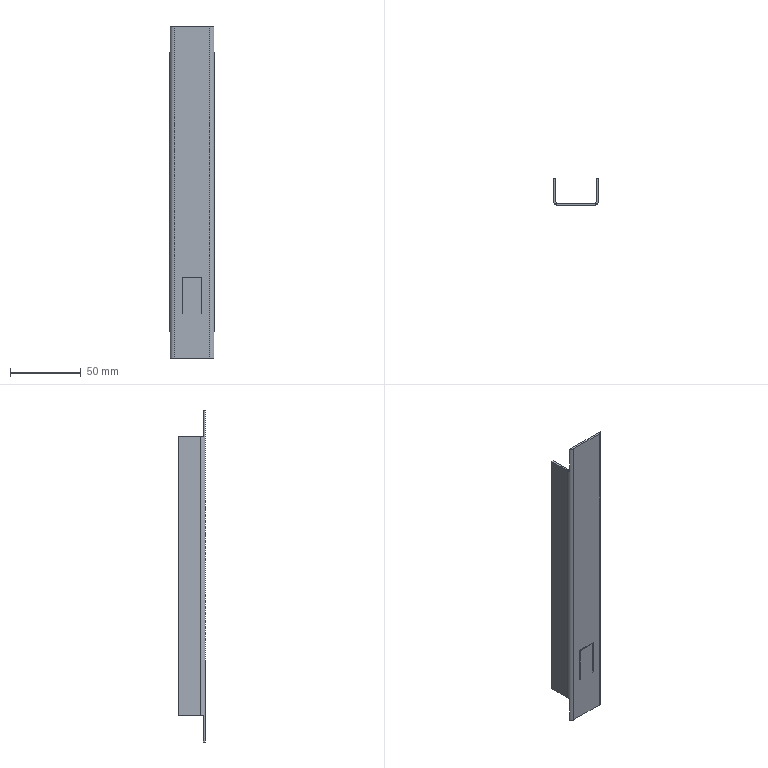Part | SolidWorks | features ICE 2, Extrusion 1 | 1 solid | 26 faces | box 31.75 x 19.05 x 234.95 mm | volume 20710 mm3 | plane 22 | cylinder 4 | commonest cylinder face diameters 3.2 x2 6.4 x2
STEP:
#1=CARTESIAN_POINT('',(31.261,1.5,234.95));
#2=VERTEX_POINT('',#1);
#3=CARTESIAN_POINT('',(0.4889,1.5,234.95));
#4=VERTEX_POINT('',#3);
#5=CARTESIAN_POINT('',(3.1,1.5,234.95));
#6=DIRECTION('',(-1.,0.,0.));
#7=VECTOR('',#6,1000.);
#8=LINE('',#5,#7);
#9=EDGE_CURVE('',#2,#4,#8,.T.);
#10=ORIENTED_EDGE('',*,*,#9,.F.);
#11=CARTESIAN_POINT('',(31.261,1.5,215.9));
#12=VERTEX_POINT('',#11);
#13=CARTESIAN_POINT('',(31.261,1.5,234.95));
#14=DIRECTION('',(0.,0.,-1.));
#15=VECTOR('',#14,1000.);
#16=LINE('',#13,#15);
#17=EDGE_CURVE('',#2,#12,#16,.T.);
#18=ORIENTED_EDGE('',*,*,#17,.T.);
#19=CARTESIAN_POINT('',(28.65,1.5,215.9));
#20=VERTEX_POINT('',#19);
#21=CARTESIAN_POINT('',(31.75,1.5,215.9));
#22=DIRECTION('',(-1.,0.,0.));
#23=VECTOR('',#22,1000.);
#24=LINE('',#21,#23);
#25=EDGE_CURVE('',#12,#20,#24,.T.);
#26=ORIENTED_EDGE('',*,*,#25,.T.);
#27=CARTESIAN_POINT('',(28.65,1.5,19.05));
#28=VERTEX_POINT('',#27);
#29=CARTESIAN_POINT('',(28.65,1.5,234.95));
#30=DIRECTION('',(0.,0.,-1.));
#31=VECTOR('',#30,1000.);
#32=LINE('',#29,#31);
#33=EDGE_CURVE('',#20,#28,#32,.T.);
#34=ORIENTED_EDGE('',*,*,#33,.T.);
#35=CARTESIAN_POINT('',(31.261,1.5,19.05));
#36=VERTEX_POINT('',#35);
#37=CARTESIAN_POINT('',(31.75,1.5,19.05));
#38=DIRECTION('',(-1.,0.,0.));
#39=VECTOR('',#38,1000.);
#40=LINE('',#37,#39);
#41=EDGE_CURVE('',#36,#28,#40,.T.);
#42=ORIENTED_EDGE('',*,*,#41,.F.);
#43=CARTESIAN_POINT('',(31.261,1.5,0.));
#44=VERTEX_POINT('',#43);
#45=CARTESIAN_POINT('',(31.261,1.5,234.95));
#46=DIRECTION('',(0.,0.,-1.));
#47=VECTOR('',#46,1000.);
#48=LINE('',#45,#47);
#49=EDGE_CURVE('',#36,#44,#48,.T.);
#50=ORIENTED_EDGE('',*,*,#49,.T.);
#51=CARTESIAN_POINT('',(0.4889,1.5,0.));
#52=VERTEX_POINT('',#51);
#53=CARTESIAN_POINT('',(3.1,1.5,0.));
#54=DIRECTION('',(-1.,0.,0.));
#55=VECTOR('',#54,1000.);
#56=LINE('',#53,#55);
#57=EDGE_CURVE('',#44,#52,#56,.T.);
#58=ORIENTED_EDGE('',*,*,#57,.T.);
#59=CARTESIAN_POINT('',(0.4889,1.5,19.05));
#60=VERTEX_POINT('',#59);
#61=CARTESIAN_POINT('',(0.4889,1.5,234.95));
#62=DIRECTION('',(0.,0.,1.));
#63=VECTOR('',#62,1000.);
#64=LINE('',#61,#63);
#65=EDGE_CURVE('',#52,#60,#64,.T.);
#66=ORIENTED_EDGE('',*,*,#65,.T.);
#67=CARTESIAN_POINT('',(3.1,1.5,19.05));
#68=VERTEX_POINT('',#67);
#69=CARTESIAN_POINT('',(31.75,1.5,19.05));
#70=DIRECTION('',(-1.,0.,0.));
#71=VECTOR('',#70,1000.);
#72=LINE('',#69,#71);
#73=EDGE_CURVE('',#68,#60,#72,.T.);
#74=ORIENTED_EDGE('',*,*,#73,.F.);
#75=CARTESIAN_POINT('',(3.1,1.5,215.9));
#76=VERTEX_POINT('',#75);
#77=CARTESIAN_POINT('',(3.1,1.5,234.95));
#78=DIRECTION('',(0.,0.,-1.));
#79=VECTOR('',#78,1000.);
#80=LINE('',#77,#79);
#81=EDGE_CURVE('',#76,#68,#80,.T.);
#82=ORIENTED_EDGE('',*,*,#81,.F.);
#83=CARTESIAN_POINT('',(0.4889,1.5,215.9));
#84=VERTEX_POINT('',#83);
#85=CARTESIAN_POINT('',(31.75,1.5,215.9));
#86=DIRECTION('',(-1.,0.,0.));
#87=VECTOR('',#86,1000.);
#88=LINE('',#85,#87);
#89=EDGE_CURVE('',#76,#84,#88,.T.);
#90=ORIENTED_EDGE('',*,*,#89,.T.);
#91=CARTESIAN_POINT('',(0.4889,1.5,234.95));
#92=DIRECTION('',(0.,0.,1.));
#93=VECTOR('',#92,1000.);
#94=LINE('',#91,#93);
#95=EDGE_CURVE('',#84,#4,#94,.T.);
#96=ORIENTED_EDGE('',*,*,#95,.T.);
#97=EDGE_LOOP('',(#10,#18,#26,#34,#42,#50,#58,#66,#74,#82,#90,#96));
#98=FACE_OUTER_BOUND('',#97,.T.);
#99=CARTESIAN_POINT('',(9.428,1.5,31.75));
#100=VERTEX_POINT('',#99);
#101=CARTESIAN_POINT('',(8.928,1.5,31.75));
#102=VERTEX_POINT('',#101);
#103=CARTESIAN_POINT('',(3.1,1.5,31.75));
#104=DIRECTION('',(-1.,0.,0.));
#105=VECTOR('',#104,1000.);
#106=LINE('',#103,#105);
#107=EDGE_CURVE('',#100,#102,#106,.T.);
#108=ORIENTED_EDGE('',*,*,#107,.F.);
#109=CARTESIAN_POINT('',(9.428,1.5,56.65));
#110=VERTEX_POINT('',#109);
#111=CARTESIAN_POINT('',(9.428,1.5,234.95));
#112=DIRECTION('',(0.,0.,-1.));
#113=VECTOR('',#112,1000.);
#114=LINE('',#111,#113);
#115=EDGE_CURVE('',#110,#100,#114,.T.);
#116=ORIENTED_EDGE('',*,*,#115,.F.);
#117=CARTESIAN_POINT('',(22.322,1.5,56.65));
#118=VERTEX_POINT('',#117);
#119=CARTESIAN_POINT('',(3.1,1.5,56.65));
#120=DIRECTION('',(-1.,0.,0.));
#121=VECTOR('',#120,1000.);
#122=LINE('',#119,#121);
#123=EDGE_CURVE('',#118,#110,#122,.T.);
#124=ORIENTED_EDGE('',*,*,#123,.F.);
#125=CARTESIAN_POINT('',(22.322,1.5,31.75));
#126=VERTEX_POINT('',#125);
#127=CARTESIAN_POINT('',(22.322,1.5,234.95));
#128=DIRECTION('',(0.,0.,1.));
#129=VECTOR('',#128,1000.);
#130=LINE('',#127,#129);
#131=EDGE_CURVE('',#126,#118,#130,.T.);
#132=ORIENTED_EDGE('',*,*,#131,.F.);
#133=CARTESIAN_POINT('',(22.822,1.5,31.75));
#134=VERTEX_POINT('',#133);
#135=CARTESIAN_POINT('',(3.1,1.5,31.75));
#136=DIRECTION('',(-1.,0.,0.));
#137=VECTOR('',#136,1000.);
#138=LINE('',#135,#137);
#139=EDGE_CURVE('',#134,#126,#138,.T.);
#140=ORIENTED_EDGE('',*,*,#139,.F.);
#141=CARTESIAN_POINT('',(22.822,1.5,57.15));
#142=VERTEX_POINT('',#141);
#143=CARTESIAN_POINT('',(22.822,1.5,234.95));
#144=DIRECTION('',(0.,0.,-1.));
#145=VECTOR('',#144,1000.);
#146=LINE('',#143,#145);
#147=EDGE_CURVE('',#142,#134,#146,.T.);
#148=ORIENTED_EDGE('',*,*,#147,.F.);
#149=CARTESIAN_POINT('',(8.928,1.5,57.15));
#150=VERTEX_POINT('',#149);
#151=CARTESIAN_POINT('',(3.1,1.5,57.15));
#152=DIRECTION('',(1.,0.,0.));
#153=VECTOR('',#152,1000.);
#154=LINE('',#151,#153);
#155=EDGE_CURVE('',#150,#142,#154,.T.);
#156=ORIENTED_EDGE('',*,*,#155,.F.);
#157=CARTESIAN_POINT('',(8.928,1.5,234.95));
#158=DIRECTION('',(0.,0.,1.));
#159=VECTOR('',#158,1000.);
#160=LINE('',#157,#159);
#161=EDGE_CURVE('',#102,#150,#160,.T.);
#162=ORIENTED_EDGE('',*,*,#161,.F.);
#163=EDGE_LOOP('',(#108,#116,#124,#132,#140,#148,#156,#162));
#164=FACE_BOUND('',#163,.T.);
#165=CARTESIAN_POINT('',(3.1,1.5,234.95));
#166=DIRECTION('',(0.,-1.,0.));
#167=DIRECTION('',(0.,0.,-1.));
#168=AXIS2_PLACEMENT_3D('',#165,#166,#167);
#169=PLANE('',#168);
#170=ADVANCED_FACE('',(#98,#164),#169,.F.);
#171=CARTESIAN_POINT('',(3.2,0.,0.));
#172=VERTEX_POINT('',#171);
#173=CARTESIAN_POINT('',(28.55,0.,0.));
#174=VERTEX_POINT('',#173);
#175=CARTESIAN_POINT('',(3.2,0.,0.));
#176=DIRECTION('',(1.,0.,0.));
#177=VECTOR('',#176,1000.);
#178=LINE('',#175,#177);
#179=EDGE_CURVE('',#172,#174,#178,.T.);
#180=ORIENTED_EDGE('',*,*,#179,.T.);
#181=CARTESIAN_POINT('',(28.55,0.,234.95));
#182=VERTEX_POINT('',#181);
#183=CARTESIAN_POINT('',(28.55,0.,234.95));
#184=DIRECTION('',(0.,0.,-1.));
#185=VECTOR('',#184,1000.);
#186=LINE('',#183,#185);
#187=EDGE_CURVE('',#182,#174,#186,.T.);
#188=ORIENTED_EDGE('',*,*,#187,.F.);
#189=CARTESIAN_POINT('',(3.2,0.,234.95));
#190=VERTEX_POINT('',#189);
#191=CARTESIAN_POINT('',(3.2,0.,234.95));
#192=DIRECTION('',(1.,0.,0.));
#193=VECTOR('',#192,1000.);
#194=LINE('',#191,#193);
#195=EDGE_CURVE('',#190,#182,#194,.T.);
#196=ORIENTED_EDGE('',*,*,#195,.F.);
#197=CARTESIAN_POINT('',(3.2,0.,234.95));
#198=DIRECTION('',(0.,0.,-1.));
#199=VECTOR('',#198,1000.);
#200=LINE('',#197,#199);
#201=EDGE_CURVE('',#190,#172,#200,.T.);
#202=ORIENTED_EDGE('',*,*,#201,.T.);
#203=EDGE_LOOP('',(#180,#188,#196,#202));
#204=FACE_OUTER_BOUND('',#203,.T.);
#205=CARTESIAN_POINT('',(9.428,0.,31.75));
#206=VERTEX_POINT('',#205);
#207=CARTESIAN_POINT('',(8.928,0.,31.75));
#208=VERTEX_POINT('',#207);
#209=CARTESIAN_POINT('',(9.428,0.,31.75));
#210=DIRECTION('',(-1.,0.,0.));
#211=VECTOR('',#210,1000.);
#212=LINE('',#209,#211);
#213=EDGE_CURVE('',#206,#208,#212,.T.);
#214=ORIENTED_EDGE('',*,*,#213,.T.);
#215=CARTESIAN_POINT('',(8.928,0.,57.15));
#216=VERTEX_POINT('',#215);
#217=CARTESIAN_POINT('',(8.928,0.,31.75));
#218=DIRECTION('',(0.,0.,1.));
#219=VECTOR('',#218,1000.);
#220=LINE('',#217,#219);
#221=EDGE_CURVE('',#208,#216,#220,.T.);
#222=ORIENTED_EDGE('',*,*,#221,.T.);
#223=CARTESIAN_POINT('',(22.822,0.,57.15));
#224=VERTEX_POINT('',#223);
#225=CARTESIAN_POINT('',(22.822,0.,57.15));
#226=DIRECTION('',(1.,0.,0.));
#227=VECTOR('',#226,1000.);
#228=LINE('',#225,#227);
#229=EDGE_CURVE('',#216,#224,#228,.T.);
#230=ORIENTED_EDGE('',*,*,#229,.T.);
#231=CARTESIAN_POINT('',(22.822,0.,31.75));
#232=VERTEX_POINT('',#231);
#233=CARTESIAN_POINT('',(22.822,0.,31.75));
#234=DIRECTION('',(0.,0.,-1.));
#235=VECTOR('',#234,1000.);
#236=LINE('',#233,#235);
#237=EDGE_CURVE('',#224,#232,#236,.T.);
#238=ORIENTED_EDGE('',*,*,#237,.T.);
#239=CARTESIAN_POINT('',(22.322,0.,31.75));
#240=VERTEX_POINT('',#239);
#241=CARTESIAN_POINT('',(22.822,0.,31.75));
#242=DIRECTION('',(-1.,0.,0.));
#243=VECTOR('',#242,1000.);
#244=LINE('',#241,#243);
#245=EDGE_CURVE('',#232,#240,#244,.T.);
#246=ORIENTED_EDGE('',*,*,#245,.T.);
#247=CARTESIAN_POINT('',(22.322,0.,56.65));
#248=VERTEX_POINT('',#247);
#249=CARTESIAN_POINT('',(22.322,0.,31.75));
#250=DIRECTION('',(0.,0.,1.));
#251=VECTOR('',#250,1000.);
#252=LINE('',#249,#251);
#253=EDGE_CURVE('',#240,#248,#252,.T.);
#254=ORIENTED_EDGE('',*,*,#253,.T.);
#255=CARTESIAN_POINT('',(9.428,0.,56.65));
#256=VERTEX_POINT('',#255);
#257=CARTESIAN_POINT('',(22.322,0.,56.65));
#258=DIRECTION('',(-1.,0.,0.));
#259=VECTOR('',#258,1000.);
#260=LINE('',#257,#259);
#261=EDGE_CURVE('',#248,#256,#260,.T.);
#262=ORIENTED_EDGE('',*,*,#261,.T.);
#263=CARTESIAN_POINT('',(9.428,0.,31.75));
#264=DIRECTION('',(0.,0.,-1.));
#265=VECTOR('',#264,1000.);
#266=LINE('',#263,#265);
#267=EDGE_CURVE('',#256,#206,#266,.T.);
#268=ORIENTED_EDGE('',*,*,#267,.T.);
#269=EDGE_LOOP('',(#214,#222,#230,#238,#246,#254,#262,#268));
#270=FACE_BOUND('',#269,.T.);
#271=CARTESIAN_POINT('',(3.2,0.,234.95));
#272=DIRECTION('',(0.,1.,0.));
#273=DIRECTION('',(0.,0.,1.));
#274=AXIS2_PLACEMENT_3D('',#271,#272,#273);
#275=PLANE('',#274);
#276=ADVANCED_FACE('',(#204,#270),#275,.F.);
#277=CARTESIAN_POINT('',(31.75,19.05,215.9));
#278=VERTEX_POINT('',#277);
#279=CARTESIAN_POINT('',(30.25,19.05,215.9));
#280=VERTEX_POINT('',#279);
#281=CARTESIAN_POINT('',(31.75,19.05,215.9));
#282=DIRECTION('',(-1.,0.,0.));
#283=VECTOR('',#282,1000.);
#284=LINE('',#281,#283);
#285=EDGE_CURVE('',#278,#280,#284,.T.);
#286=ORIENTED_EDGE('',*,*,#285,.F.);
#287=CARTESIAN_POINT('',(31.75,19.05,19.05));
#288=VERTEX_POINT('',#287);
#289=CARTESIAN_POINT('',(31.75,19.05,234.95));
#290=DIRECTION('',(0.,0.,-1.));
#291=VECTOR('',#290,1000.);
#292=LINE('',#289,#291);
#293=EDGE_CURVE('',#278,#288,#292,.T.);
#294=ORIENTED_EDGE('',*,*,#293,.T.);
#295=CARTESIAN_POINT('',(30.25,19.05,19.05));
#296=VERTEX_POINT('',#295);
#297=CARTESIAN_POINT('',(31.75,19.05,19.05));
#298=DIRECTION('',(-1.,0.,0.));
#299=VECTOR('',#298,1000.);
#300=LINE('',#297,#299);
#301=EDGE_CURVE('',#288,#296,#300,.T.);
#302=ORIENTED_EDGE('',*,*,#301,.T.);
#303=CARTESIAN_POINT('',(30.25,19.05,234.95));
#304=DIRECTION('',(0.,0.,-1.));
#305=VECTOR('',#304,1000.);
#306=LINE('',#303,#305);
#307=EDGE_CURVE('',#280,#296,#306,.T.);
#308=ORIENTED_EDGE('',*,*,#307,.F.);
#309=EDGE_LOOP('',(#286,#294,#302,#308));
#310=FACE_OUTER_BOUND('',#309,.T.);
#311=CARTESIAN_POINT('',(31.75,19.05,234.95));
#312=DIRECTION('',(0.,-1.,0.));
#313=DIRECTION('',(0.,0.,-1.));
#314=AXIS2_PLACEMENT_3D('',#311,#312,#313);
#315=PLANE('',#314);
#316=ADVANCED_FACE('',(#310),#315,.F.);
#317=CARTESIAN_POINT('',(30.25,3.1,215.9));
#318=VERTEX_POINT('',#317);
#319=CARTESIAN_POINT('',(30.25,3.1,215.9));
#320=DIRECTION('',(0.,-1.,0.));
#321=VECTOR('',#320,1000.);
#322=LINE('',#319,#321);
#323=EDGE_CURVE('',#280,#318,#322,.T.);
#324=ORIENTED_EDGE('',*,*,#323,.F.);
#325=ORIENTED_EDGE('',*,*,#307,.T.);
#326=CARTESIAN_POINT('',(30.25,3.1,19.05));
#327=VERTEX_POINT('',#326);
#328=CARTESIAN_POINT('',(30.25,3.1,19.05));
#329=DIRECTION('',(0.,1.,0.));
#330=VECTOR('',#329,1000.);
#331=LINE('',#328,#330);
#332=EDGE_CURVE('',#327,#296,#331,.T.);
#333=ORIENTED_EDGE('',*,*,#332,.F.);
#334=CARTESIAN_POINT('',(30.25,3.1,234.95));
#335=DIRECTION('',(0.,0.,-1.));
#336=VECTOR('',#335,1000.);
#337=LINE('',#334,#336);
#338=EDGE_CURVE('',#318,#327,#337,.T.);
#339=ORIENTED_EDGE('',*,*,#338,.F.);
#340=EDGE_LOOP('',(#324,#325,#333,#339));
#341=FACE_OUTER_BOUND('',#340,.T.);
#342=CARTESIAN_POINT('',(30.25,3.1,234.95));
#343=DIRECTION('',(1.,0.,0.));
#344=DIRECTION('',(0.,1.,0.));
#345=AXIS2_PLACEMENT_3D('',#342,#343,#344);
#346=PLANE('',#345);
#347=ADVANCED_FACE('',(#341),#346,.F.);
#348=CARTESIAN_POINT('',(28.65,3.1,215.9));
#349=DIRECTION('',(0.,0.,-1.));
#350=DIRECTION('',(1.,0.,0.));
#351=AXIS2_PLACEMENT_3D('',#348,#349,#350);
#352=CIRCLE('',#351,1.6);
#353=EDGE_CURVE('',#318,#20,#352,.T.);
#354=ORIENTED_EDGE('',*,*,#353,.F.);
#355=ORIENTED_EDGE('',*,*,#338,.T.);
#356=CARTESIAN_POINT('',(28.65,3.1,19.05));
#357=DIRECTION('',(0.,0.,1.));
#358=DIRECTION('',(0.,1.,0.));
#359=AXIS2_PLACEMENT_3D('',#356,#357,#358);
#360=CIRCLE('',#359,1.6);
#361=EDGE_CURVE('',#28,#327,#360,.T.);
#362=ORIENTED_EDGE('',*,*,#361,.F.);
#363=ORIENTED_EDGE('',*,*,#33,.F.);
#364=EDGE_LOOP('',(#354,#355,#362,#363));
#365=FACE_OUTER_BOUND('',#364,.T.);
#366=CARTESIAN_POINT('',(28.65,3.1,234.95));
#367=DIRECTION('',(0.,0.,-1.));
#368=DIRECTION('',(-1.,0.,0.));
#369=AXIS2_PLACEMENT_3D('',#366,#367,#368);
#370=CYLINDRICAL_SURFACE('',#369,1.6);
#371=ADVANCED_FACE('',(#365),#370,.F.);
#372=CARTESIAN_POINT('',(1.5,3.1,215.9));
#373=VERTEX_POINT('',#372);
#374=CARTESIAN_POINT('',(3.1,3.1,215.9));
#375=DIRECTION('',(0.,0.,-1.));
#376=DIRECTION('',(1.,0.,0.));
#377=AXIS2_PLACEMENT_3D('',#374,#375,#376);
#378=CIRCLE('',#377,1.6);
#379=EDGE_CURVE('',#76,#373,#378,.T.);
#380=ORIENTED_EDGE('',*,*,#379,.F.);
#381=ORIENTED_EDGE('',*,*,#81,.T.);
#382=CARTESIAN_POINT('',(1.5,3.1,19.05));
#383=VERTEX_POINT('',#382);
#384=CARTESIAN_POINT('',(3.1,3.1,19.05));
#385=DIRECTION('',(0.,0.,1.));
#386=DIRECTION('',(0.,1.,0.));
#387=AXIS2_PLACEMENT_3D('',#384,#385,#386);
#388=CIRCLE('',#387,1.6);
#389=EDGE_CURVE('',#383,#68,#388,.T.);
#390=ORIENTED_EDGE('',*,*,#389,.F.);
#391=CARTESIAN_POINT('',(1.5,3.1,234.95));
#392=DIRECTION('',(0.,0.,-1.));
#393=VECTOR('',#392,1000.);
#394=LINE('',#391,#393);
#395=EDGE_CURVE('',#373,#383,#394,.T.);
#396=ORIENTED_EDGE('',*,*,#395,.F.);
#397=EDGE_LOOP('',(#380,#381,#390,#396));
#398=FACE_OUTER_BOUND('',#397,.T.);
#399=CARTESIAN_POINT('',(3.1,3.1,234.95));
#400=DIRECTION('',(0.,0.,-1.));
#401=DIRECTION('',(-1.,0.,0.));
#402=AXIS2_PLACEMENT_3D('',#399,#400,#401);
#403=CYLINDRICAL_SURFACE('',#402,1.6);
#404=ADVANCED_FACE('',(#398),#403,.F.);
#405=CARTESIAN_POINT('',(1.5,19.05,215.9));
#406=VERTEX_POINT('',#405);
#407=CARTESIAN_POINT('',(1.5,3.1,215.9));
#408=DIRECTION('',(0.,1.,0.));
#409=VECTOR('',#408,1000.);
#410=LINE('',#407,#409);
#411=EDGE_CURVE('',#373,#406,#410,.T.);
#412=ORIENTED_EDGE('',*,*,#411,.F.);
#413=ORIENTED_EDGE('',*,*,#395,.T.);
#414=CARTESIAN_POINT('',(1.5,19.05,19.05));
#415=VERTEX_POINT('',#414);
#416=CARTESIAN_POINT('',(1.5,3.1,19.05));
#417=DIRECTION('',(0.,-1.,0.));
#418=VECTOR('',#417,1000.);
#419=LINE('',#416,#418);
#420=EDGE_CURVE('',#415,#383,#419,.T.);
#421=ORIENTED_EDGE('',*,*,#420,.F.);
#422=CARTESIAN_POINT('',(1.5,19.05,234.95));
#423=DIRECTION('',(0.,0.,-1.));
#424=VECTOR('',#423,1000.);
#425=LINE('',#422,#424);
#426=EDGE_CURVE('',#406,#415,#425,.T.);
#427=ORIENTED_EDGE('',*,*,#426,.F.);
#428=EDGE_LOOP('',(#412,#413,#421,#427));
#429=FACE_OUTER_BOUND('',#428,.T.);
#430=CARTESIAN_POINT('',(1.5,3.1,234.95));
#431=DIRECTION('',(-1.,0.,0.));
#432=DIRECTION('',(0.,-1.,0.));
#433=AXIS2_PLACEMENT_3D('',#430,#431,#432);
#434=PLANE('',#433);
#435=ADVANCED_FACE('',(#429),#434,.F.);
#436=CARTESIAN_POINT('',(0.,19.05,215.9));
#437=VERTEX_POINT('',#436);
#438=CARTESIAN_POINT('',(31.75,19.05,215.9));
#439=DIRECTION('',(-1.,0.,0.));
#440=VECTOR('',#439,1000.);
#441=LINE('',#438,#440);
#442=EDGE_CURVE('',#406,#437,#441,.T.);
#443=ORIENTED_EDGE('',*,*,#442,.F.);
#444=ORIENTED_EDGE('',*,*,#426,.T.);
#445=CARTESIAN_POINT('',(0.,19.05,19.05));
#446=VERTEX_POINT('',#445);
#447=CARTESIAN_POINT('',(31.75,19.05,19.05));
#448=DIRECTION('',(-1.,0.,0.));
#449=VECTOR('',#448,1000.);
#450=LINE('',#447,#449);
#451=EDGE_CURVE('',#415,#446,#450,.T.);
#452=ORIENTED_EDGE('',*,*,#451,.T.);
#453=CARTESIAN_POINT('',(0.,19.05,234.95));
#454=DIRECTION('',(0.,0.,-1.));
#455=VECTOR('',#454,1000.);
#456=LINE('',#453,#455);
#457=EDGE_CURVE('',#437,#446,#456,.T.);
#458=ORIENTED_EDGE('',*,*,#457,.F.);
#459=EDGE_LOOP('',(#443,#444,#452,#458));
#460=FACE_OUTER_BOUND('',#459,.T.);
#461=CARTESIAN_POINT('',(1.5,19.05,234.95));
#462=DIRECTION('',(0.,-1.,0.));
#463=DIRECTION('',(0.,0.,-1.));
#464=AXIS2_PLACEMENT_3D('',#461,#462,#463);
#465=PLANE('',#464);
#466=ADVANCED_FACE('',(#460),#465,.F.);
#467=CARTESIAN_POINT('',(0.,3.2,215.9));
#468=VERTEX_POINT('',#467);
#469=CARTESIAN_POINT('',(0.,1.5,215.9));
#470=DIRECTION('',(0.,1.,0.));
#471=VECTOR('',#470,1000.);
#472=LINE('',#469,#471);
#473=EDGE_CURVE('',#468,#437,#472,.T.);
#474=ORIENTED_EDGE('',*,*,#473,.T.);
#475=ORIENTED_EDGE('',*,*,#457,.T.);
#476=CARTESIAN_POINT('',(0.,3.2,19.05));
#477=VERTEX_POINT('',#476);
#478=CARTESIAN_POINT('',(0.,1.5,19.05));
#479=DIRECTION('',(0.,-1.,0.));
#480=VECTOR('',#479,1000.);
#481=LINE('',#478,#480);
#482=EDGE_CURVE('',#446,#477,#481,.T.);
#483=ORIENTED_EDGE('',*,*,#482,.T.);
#484=CARTESIAN_POINT('',(0.,3.2,234.95));
#485=DIRECTION('',(0.,0.,-1.));
#486=VECTOR('',#485,1000.);
#487=LINE('',#484,#486);
#488=EDGE_CURVE('',#468,#477,#487,.T.);
#489=ORIENTED_EDGE('',*,*,#488,.F.);
#490=EDGE_LOOP('',(#474,#475,#483,#489));
#491=FACE_OUTER_BOUND('',#490,.T.);
#492=CARTESIAN_POINT('',(0.,3.2,234.95));
#493=DIRECTION('',(1.,0.,0.));
#494=DIRECTION('',(0.,0.,-1.));
#495=AXIS2_PLACEMENT_3D('',#492,#493,#494);
#496=PLANE('',#495);
#497=ADVANCED_FACE('',(#491),#496,.F.);
#498=ORIENTED_EDGE('',*,*,#95,.F.);
#499=CARTESIAN_POINT('',(3.2,3.2,215.9));
#500=DIRECTION('',(0.,0.,1.));
#501=DIRECTION('',(1.,0.,0.));
#502=AXIS2_PLACEMENT_3D('',#499,#500,#501);
#503=CIRCLE('',#502,3.2);
#504=EDGE_CURVE('',#468,#84,#503,.T.);
#505=ORIENTED_EDGE('',*,*,#504,.F.);
#506=ORIENTED_EDGE('',*,*,#488,.T.);
#507=CARTESIAN_POINT('',(3.2,3.2,19.05));
#508=DIRECTION('',(0.,0.,-1.));
#509=DIRECTION('',(0.,1.,0.));
#510=AXIS2_PLACEMENT_3D('',#507,#508,#509);
#511=CIRCLE('',#510,3.2);
#512=EDGE_CURVE('',#60,#477,#511,.T.);
#513=ORIENTED_EDGE('',*,*,#512,.F.);
#514=ORIENTED_EDGE('',*,*,#65,.F.);
#515=CARTESIAN_POINT('',(3.2,3.2,0.));
#516=DIRECTION('',(0.,0.,1.));
#517=DIRECTION('',(1.,0.,0.));
#518=AXIS2_PLACEMENT_3D('',#515,#516,#517);
#519=CIRCLE('',#518,3.2);
#520=EDGE_CURVE('',#52,#172,#519,.T.);
#521=ORIENTED_EDGE('',*,*,#520,.T.);
#522=ORIENTED_EDGE('',*,*,#201,.F.);
#523=CARTESIAN_POINT('',(3.2,3.2,234.95));
#524=DIRECTION('',(0.,0.,1.));
#525=DIRECTION('',(1.,0.,0.));
#526=AXIS2_PLACEMENT_3D('',#523,#524,#525);
#527=CIRCLE('',#526,3.2);
#528=EDGE_CURVE('',#4,#190,#527,.T.);
#529=ORIENTED_EDGE('',*,*,#528,.F.);
#530=EDGE_LOOP('',(#498,#505,#506,#513,#514,#521,#522,#529));
#531=FACE_OUTER_BOUND('',#530,.T.);
#532=CARTESIAN_POINT('',(3.2,3.2,234.95));
#533=DIRECTION('',(0.,0.,-1.));
#534=DIRECTION('',(-1.,0.,0.));
#535=AXIS2_PLACEMENT_3D('',#532,#533,#534);
#536=CYLINDRICAL_SURFACE('',#535,3.2);
#537=ADVANCED_FACE('',(#531),#536,.T.);
#538=ORIENTED_EDGE('',*,*,#17,.F.);
#539=CARTESIAN_POINT('',(28.55,3.2,234.95));
#540=DIRECTION('',(0.,0.,1.));
#541=DIRECTION('',(-1.,0.,0.));
#542=AXIS2_PLACEMENT_3D('',#539,#540,#541);
#543=CIRCLE('',#542,3.2);
#544=EDGE_CURVE('',#182,#2,#543,.T.);
#545=ORIENTED_EDGE('',*,*,#544,.F.);
#546=ORIENTED_EDGE('',*,*,#187,.T.);
#547=CARTESIAN_POINT('',(28.55,3.2,0.));
#548=DIRECTION('',(0.,0.,1.));
#549=DIRECTION('',(-1.,0.,0.));
#550=AXIS2_PLACEMENT_3D('',#547,#548,#549);
#551=CIRCLE('',#550,3.2);
#552=EDGE_CURVE('',#174,#44,#551,.T.);
#553=ORIENTED_EDGE('',*,*,#552,.T.);
#554=ORIENTED_EDGE('',*,*,#49,.F.);
#555=CARTESIAN_POINT('',(31.75,3.2,19.05));
#556=VERTEX_POINT('',#555);
#557=CARTESIAN_POINT('',(28.55,3.2,19.05));
#558=DIRECTION('',(0.,0.,-1.));
#559=DIRECTION('',(0.,1.,0.));
#560=AXIS2_PLACEMENT_3D('',#557,#558,#559);
#561=CIRCLE('',#560,3.2);
#562=EDGE_CURVE('',#556,#36,#561,.T.);
#563=ORIENTED_EDGE('',*,*,#562,.F.);
#564=CARTESIAN_POINT('',(31.75,3.2,215.9));
#565=VERTEX_POINT('',#564);
#566=CARTESIAN_POINT('',(31.75,3.2,234.95));
#567=DIRECTION('',(0.,0.,-1.));
#568=VECTOR('',#567,1000.);
#569=LINE('',#566,#568);
#570=EDGE_CURVE('',#565,#556,#569,.T.);
#571=ORIENTED_EDGE('',*,*,#570,.F.);
#572=CARTESIAN_POINT('',(28.55,3.2,215.9));
#573=DIRECTION('',(0.,0.,1.));
#574=DIRECTION('',(1.,0.,0.));
#575=AXIS2_PLACEMENT_3D('',#572,#573,#574);
#576=CIRCLE('',#575,3.2);
#577=EDGE_CURVE('',#12,#565,#576,.T.);
#578=ORIENTED_EDGE('',*,*,#577,.F.);
#579=EDGE_LOOP('',(#538,#545,#546,#553,#554,#563,#571,#578));
#580=FACE_OUTER_BOUND('',#579,.T.);
#581=CARTESIAN_POINT('',(28.55,3.2,234.95));
#582=DIRECTION('',(0.,0.,-1.));
#583=DIRECTION('',(-1.,0.,0.));
#584=AXIS2_PLACEMENT_3D('',#581,#582,#583);
#585=CYLINDRICAL_SURFACE('',#584,3.2);
#586=ADVANCED_FACE('',(#580),#585,.T.);
#587=CARTESIAN_POINT('',(31.75,1.5,215.9));
#588=DIRECTION('',(0.,1.,0.));
#589=VECTOR('',#588,1000.);
#590=LINE('',#587,#589);
#591=EDGE_CURVE('',#565,#278,#590,.T.);
#592=ORIENTED_EDGE('',*,*,#591,.F.);
#593=ORIENTED_EDGE('',*,*,#570,.T.);
#594=CARTESIAN_POINT('',(31.75,1.5,19.05));
#595=DIRECTION('',(0.,-1.,0.));
#596=VECTOR('',#595,1000.);
#597=LINE('',#594,#596);
#598=EDGE_CURVE('',#288,#556,#597,.T.);
#599=ORIENTED_EDGE('',*,*,#598,.F.);
#600=ORIENTED_EDGE('',*,*,#293,.F.);
#601=EDGE_LOOP('',(#592,#593,#599,#600));
#602=FACE_OUTER_BOUND('',#601,.T.);
#603=CARTESIAN_POINT('',(31.75,3.2,234.95));
#604=DIRECTION('',(-1.,0.,0.));
#605=DIRECTION('',(0.,0.,1.));
#606=AXIS2_PLACEMENT_3D('',#603,#604,#605);
#607=PLANE('',#606);
#608=ADVANCED_FACE('',(#602),#607,.F.);
#609=ORIENTED_EDGE('',*,*,#544,.T.);
#610=ORIENTED_EDGE('',*,*,#9,.T.);
#611=ORIENTED_EDGE('',*,*,#528,.T.);
#612=ORIENTED_EDGE('',*,*,#195,.T.);
#613=EDGE_LOOP('',(#609,#610,#611,#612));
#614=FACE_OUTER_BOUND('',#613,.T.);
#615=CARTESIAN_POINT('',(28.65,3.1,234.95));
#616=DIRECTION('',(0.,0.,1.));
#617=DIRECTION('',(1.,0.,0.));
#618=AXIS2_PLACEMENT_3D('',#615,#616,#617);
#619=PLANE('',#618);
#620=ADVANCED_FACE('',(#614),#619,.T.);
#621=ORIENTED_EDGE('',*,*,#57,.F.);
#622=ORIENTED_EDGE('',*,*,#552,.F.);
#623=ORIENTED_EDGE('',*,*,#179,.F.);
#624=ORIENTED_EDGE('',*,*,#520,.F.);
#625=EDGE_LOOP('',(#621,#622,#623,#624));
#626=FACE_OUTER_BOUND('',#625,.T.);
#627=CARTESIAN_POINT('',(28.65,3.1,0.));
#628=DIRECTION('',(0.,0.,1.));
#629=DIRECTION('',(1.,0.,0.));
#630=AXIS2_PLACEMENT_3D('',#627,#628,#629);
#631=PLANE('',#630);
#632=ADVANCED_FACE('',(#626),#631,.F.);
#633=ORIENTED_EDGE('',*,*,#389,.T.);
#634=ORIENTED_EDGE('',*,*,#73,.T.);
#635=ORIENTED_EDGE('',*,*,#512,.T.);
#636=ORIENTED_EDGE('',*,*,#482,.F.);
#637=ORIENTED_EDGE('',*,*,#451,.F.);
#638=ORIENTED_EDGE('',*,*,#420,.T.);
#639=EDGE_LOOP('',(#633,#634,#635,#636,#637,#638));
#640=FACE_OUTER_BOUND('',#639,.T.);
#641=CARTESIAN_POINT('',(31.75,1.5,19.05));
#642=DIRECTION('',(0.,0.,-1.));
#643=DIRECTION('',(0.,1.,0.));
#644=AXIS2_PLACEMENT_3D('',#641,#642,#643);
#645=PLANE('',#644);
#646=ADVANCED_FACE('',(#640),#645,.T.);
#647=ORIENTED_EDGE('',*,*,#332,.T.);
#648=ORIENTED_EDGE('',*,*,#301,.F.);
#649=ORIENTED_EDGE('',*,*,#598,.T.);
#650=ORIENTED_EDGE('',*,*,#562,.T.);
#651=ORIENTED_EDGE('',*,*,#41,.T.);
#652=ORIENTED_EDGE('',*,*,#361,.T.);
#653=EDGE_LOOP('',(#647,#648,#649,#650,#651,#652));
#654=FACE_OUTER_BOUND('',#653,.T.);
#655=CARTESIAN_POINT('',(31.75,1.5,19.05));
#656=DIRECTION('',(0.,0.,-1.));
#657=DIRECTION('',(0.,1.,0.));
#658=AXIS2_PLACEMENT_3D('',#655,#656,#657);
#659=PLANE('',#658);
#660=ADVANCED_FACE('',(#654),#659,.T.);
#661=ORIENTED_EDGE('',*,*,#379,.T.);
#662=ORIENTED_EDGE('',*,*,#411,.T.);
#663=ORIENTED_EDGE('',*,*,#442,.T.);
#664=ORIENTED_EDGE('',*,*,#473,.F.);
#665=ORIENTED_EDGE('',*,*,#504,.T.);
#666=ORIENTED_EDGE('',*,*,#89,.F.);
#667=EDGE_LOOP('',(#661,#662,#663,#664,#665,#666));
#668=FACE_OUTER_BOUND('',#667,.T.);
#669=CARTESIAN_POINT('',(31.75,1.5,215.9));
#670=DIRECTION('',(0.,0.,1.));
#671=DIRECTION('',(1.,0.,0.));
#672=AXIS2_PLACEMENT_3D('',#669,#670,#671);
#673=PLANE('',#672);
#674=ADVANCED_FACE('',(#668),#673,.T.);
#675=ORIENTED_EDGE('',*,*,#323,.T.);
#676=ORIENTED_EDGE('',*,*,#353,.T.);
#677=ORIENTED_EDGE('',*,*,#25,.F.);
#678=ORIENTED_EDGE('',*,*,#577,.T.);
#679=ORIENTED_EDGE('',*,*,#591,.T.);
#680=ORIENTED_EDGE('',*,*,#285,.T.);
#681=EDGE_LOOP('',(#675,#676,#677,#678,#679,#680));
#682=FACE_OUTER_BOUND('',#681,.T.);
#683=CARTESIAN_POINT('',(31.75,1.5,215.9));
#684=DIRECTION('',(0.,0.,1.));
#685=DIRECTION('',(1.,0.,0.));
#686=AXIS2_PLACEMENT_3D('',#683,#684,#685);
#687=PLANE('',#686);
#688=ADVANCED_FACE('',(#682),#687,.T.);
#689=ORIENTED_EDGE('',*,*,#107,.T.);
#690=CARTESIAN_POINT('',(8.928,19.05,31.75));
#691=DIRECTION('',(0.,-1.,0.));
#692=VECTOR('',#691,1000.);
#693=LINE('',#690,#692);
#694=EDGE_CURVE('',#102,#208,#693,.T.);
#695=ORIENTED_EDGE('',*,*,#694,.T.);
#696=ORIENTED_EDGE('',*,*,#213,.F.);
#697=CARTESIAN_POINT('',(9.428,19.05,31.75));
#698=DIRECTION('',(0.,-1.,0.));
#699=VECTOR('',#698,1000.);
#700=LINE('',#697,#699);
#701=EDGE_CURVE('',#100,#206,#700,.T.);
#702=ORIENTED_EDGE('',*,*,#701,.F.);
#703=EDGE_LOOP('',(#689,#695,#696,#702));
#704=FACE_OUTER_BOUND('',#703,.T.);
#705=CARTESIAN_POINT('',(9.428,19.05,31.75));
#706=DIRECTION('',(0.,0.,1.));
#707=DIRECTION('',(1.,0.,0.));
#708=AXIS2_PLACEMENT_3D('',#705,#706,#707);
#709=PLANE('',#708);
#710=ADVANCED_FACE('',(#704),#709,.T.);
#711=ORIENTED_EDGE('',*,*,#161,.T.);
#712=CARTESIAN_POINT('',(8.928,19.05,57.15));
#713=DIRECTION('',(0.,-1.,0.));
#714=VECTOR('',#713,1000.);
#715=LINE('',#712,#714);
#716=EDGE_CURVE('',#150,#216,#715,.T.);
#717=ORIENTED_EDGE('',*,*,#716,.T.);
#718=ORIENTED_EDGE('',*,*,#221,.F.);
#719=ORIENTED_EDGE('',*,*,#694,.F.);
#720=EDGE_LOOP('',(#711,#717,#718,#719));
#721=FACE_OUTER_BOUND('',#720,.T.);
#722=CARTESIAN_POINT('',(8.928,19.05,31.75));
#723=DIRECTION('',(1.,0.,0.));
#724=DIRECTION('',(0.,0.,-1.));
#725=AXIS2_PLACEMENT_3D('',#722,#723,#724);
#726=PLANE('',#725);
#727=ADVANCED_FACE('',(#721),#726,.T.);
#728=ORIENTED_EDGE('',*,*,#155,.T.);
#729=CARTESIAN_POINT('',(22.822,19.05,57.15));
#730=DIRECTION('',(0.,-1.,0.));
#731=VECTOR('',#730,1000.);
#732=LINE('',#729,#731);
#733=EDGE_CURVE('',#142,#224,#732,.T.);
#734=ORIENTED_EDGE('',*,*,#733,.T.);
#735=ORIENTED_EDGE('',*,*,#229,.F.);
#736=ORIENTED_EDGE('',*,*,#716,.F.);
#737=EDGE_LOOP('',(#728,#734,#735,#736));
#738=FACE_OUTER_BOUND('',#737,.T.);
#739=CARTESIAN_POINT('',(22.822,19.05,57.15));
#740=DIRECTION('',(0.,0.,-1.));
#741=DIRECTION('',(-1.,0.,0.));
#742=AXIS2_PLACEMENT_3D('',#739,#740,#741);
#743=PLANE('',#742);
#744=ADVANCED_FACE('',(#738),#743,.T.);
#745=ORIENTED_EDGE('',*,*,#147,.T.);
#746=CARTESIAN_POINT('',(22.822,19.05,31.75));
#747=DIRECTION('',(0.,-1.,0.));
#748=VECTOR('',#747,1000.);
#749=LINE('',#746,#748);
#750=EDGE_CURVE('',#134,#232,#749,.T.);
#751=ORIENTED_EDGE('',*,*,#750,.T.);
#752=ORIENTED_EDGE('',*,*,#237,.F.);
#753=ORIENTED_EDGE('',*,*,#733,.F.);
#754=EDGE_LOOP('',(#745,#751,#752,#753));
#755=FACE_OUTER_BOUND('',#754,.T.);
#756=CARTESIAN_POINT('',(22.822,19.05,31.75));
#757=DIRECTION('',(-1.,0.,0.));
#758=DIRECTION('',(0.,0.,1.));
#759=AXIS2_PLACEMENT_3D('',#756,#757,#758);
#760=PLANE('',#759);
#761=ADVANCED_FACE('',(#755),#760,.T.);
#762=ORIENTED_EDGE('',*,*,#139,.T.);
#763=CARTESIAN_POINT('',(22.322,19.05,31.75));
#764=DIRECTION('',(0.,-1.,0.));
#765=VECTOR('',#764,1000.);
#766=LINE('',#763,#765);
#767=EDGE_CURVE('',#126,#240,#766,.T.);
#768=ORIENTED_EDGE('',*,*,#767,.T.);
#769=ORIENTED_EDGE('',*,*,#245,.F.);
#770=ORIENTED_EDGE('',*,*,#750,.F.);
#771=EDGE_LOOP('',(#762,#768,#769,#770));
#772=FACE_OUTER_BOUND('',#771,.T.);
#773=CARTESIAN_POINT('',(22.822,19.05,31.75));
#774=DIRECTION('',(0.,0.,1.));
#775=DIRECTION('',(1.,0.,0.));
#776=AXIS2_PLACEMENT_3D('',#773,#774,#775);
#777=PLANE('',#776);
#778=ADVANCED_FACE('',(#772),#777,.T.);
#779=ORIENTED_EDGE('',*,*,#131,.T.);
#780=CARTESIAN_POINT('',(22.322,19.05,56.65));
#781=DIRECTION('',(0.,-1.,0.));
#782=VECTOR('',#781,1000.);
#783=LINE('',#780,#782);
#784=EDGE_CURVE('',#118,#248,#783,.T.);
#785=ORIENTED_EDGE('',*,*,#784,.T.);
#786=ORIENTED_EDGE('',*,*,#253,.F.);
#787=ORIENTED_EDGE('',*,*,#767,.F.);
#788=EDGE_LOOP('',(#779,#785,#786,#787));
#789=FACE_OUTER_BOUND('',#788,.T.);
#790=CARTESIAN_POINT('',(22.322,19.05,31.75));
#791=DIRECTION('',(1.,0.,0.));
#792=DIRECTION('',(0.,0.,-1.));
#793=AXIS2_PLACEMENT_3D('',#790,#791,#792);
#794=PLANE('',#793);
#795=ADVANCED_FACE('',(#789),#794,.T.);
#796=ORIENTED_EDGE('',*,*,#123,.T.);
#797=CARTESIAN_POINT('',(9.428,19.05,56.65));
#798=DIRECTION('',(0.,-1.,0.));
#799=VECTOR('',#798,1000.);
#800=LINE('',#797,#799);
#801=EDGE_CURVE('',#110,#256,#800,.T.);
#802=ORIENTED_EDGE('',*,*,#801,.T.);
#803=ORIENTED_EDGE('',*,*,#261,.F.);
#804=ORIENTED_EDGE('',*,*,#784,.F.);
#805=EDGE_LOOP('',(#796,#802,#803,#804));
#806=FACE_OUTER_BOUND('',#805,.T.);
#807=CARTESIAN_POINT('',(22.322,19.05,56.65));
#808=DIRECTION('',(0.,0.,1.));
#809=DIRECTION('',(1.,0.,0.));
#810=AXIS2_PLACEMENT_3D('',#807,#808,#809);
#811=PLANE('',#810);
#812=ADVANCED_FACE('',(#806),#811,.T.);
#813=ORIENTED_EDGE('',*,*,#115,.T.);
#814=ORIENTED_EDGE('',*,*,#701,.T.);
#815=ORIENTED_EDGE('',*,*,#267,.F.);
#816=ORIENTED_EDGE('',*,*,#801,.F.);
#817=EDGE_LOOP('',(#813,#814,#815,#816));
#818=FACE_OUTER_BOUND('',#817,.T.);
#819=CARTESIAN_POINT('',(9.428,19.05,31.75));
#820=DIRECTION('',(-1.,0.,0.));
#821=DIRECTION('',(0.,0.,1.));
#822=AXIS2_PLACEMENT_3D('',#819,#820,#821);
#823=PLANE('',#822);
#824=ADVANCED_FACE('',(#818),#823,.T.);
#825=CLOSED_SHELL('',(#170,#276,#316,#347,#371,#404,#435,#466,#497,#537,#586,#608,#620,#632,#646,#660,#674,#688,#710,#727,#744,#761,#778,#795,#812,#824));
#826=MANIFOLD_SOLID_BREP('',#825);
#827=CARTESIAN_POINT('',(0.,0.,0.));
#828=DIRECTION('',(0.,0.,1.));
#829=DIRECTION('',(1.,0.,0.));
#830=AXIS2_PLACEMENT_3D('',#827,#828,#829);
#831=(LENGTH_UNIT()NAMED_UNIT(*)SI_UNIT(.MILLI.,.METRE.));
#832=UNCERTAINTY_MEASURE_WITH_UNIT(LENGTH_MEASURE(0.00001),#831,'','');
#833=(NAMED_UNIT(*)PLANE_ANGLE_UNIT()SI_UNIT($,.RADIAN.));
#834=(NAMED_UNIT(*)SI_UNIT($,.STERADIAN.)SOLID_ANGLE_UNIT());
#835=(GEOMETRIC_REPRESENTATION_CONTEXT(3)GLOBAL_UNCERTAINTY_ASSIGNED_CONTEXT((#832))GLOBAL_UNIT_ASSIGNED_CONTEXT((#831,#833,#834))REPRESENTATION_CONTEXT('',''));
#836=ADVANCED_BREP_SHAPE_REPRESENTATION('',(#826,#830),#835);